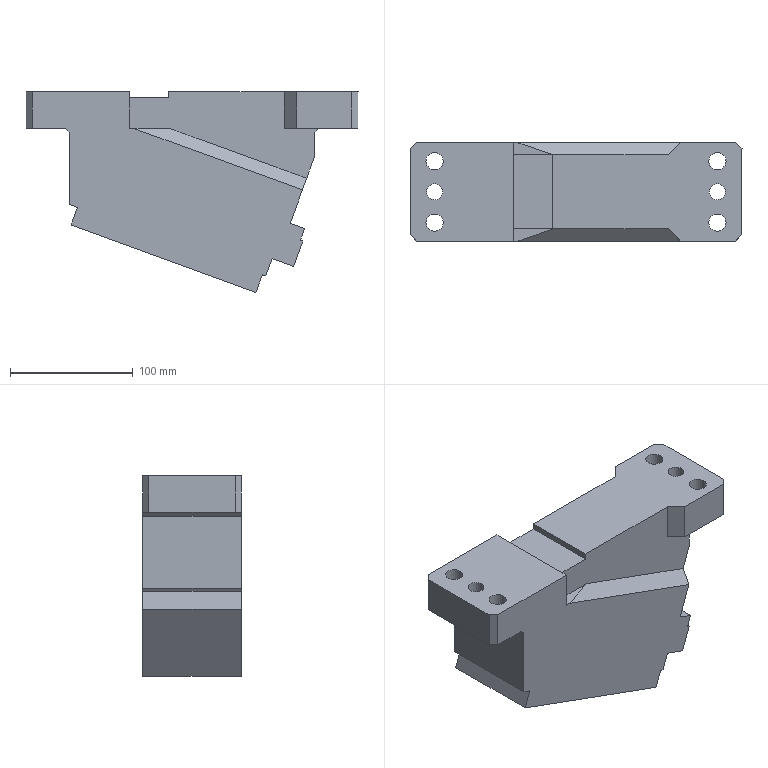Part | NX | features solid 2 | 1 solid | 55 faces | box 270 x 80 x 163.304 mm | volume 2100363 mm3 | plane 45 | cylinder 10 | commonest cylinder face diameters 14 x4 20 x4 13 x2